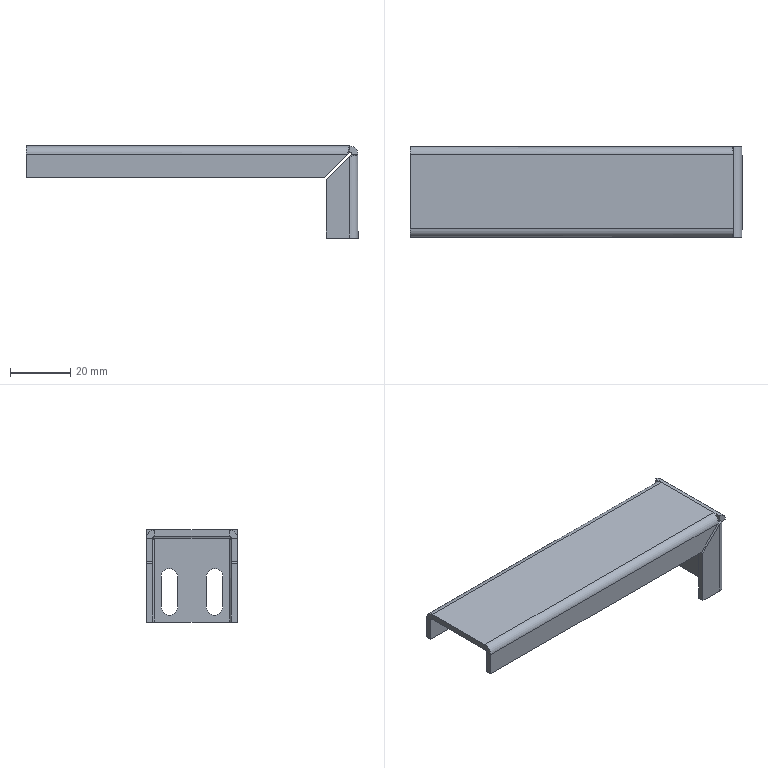Part | SolidWorks | features EdgeFlange 2, FlatPattern 1, ICE 1, SMBaseFlange 1, SheetMetal 1 | 1 solid | 60 faces | box 110 x 30 x 30.5 mm | volume 11846 mm3 | plane 40 | cylinder 16 | spline 4 | commonest cylinder face diameters 5.5 x6 1.473 x5 5.473 x5